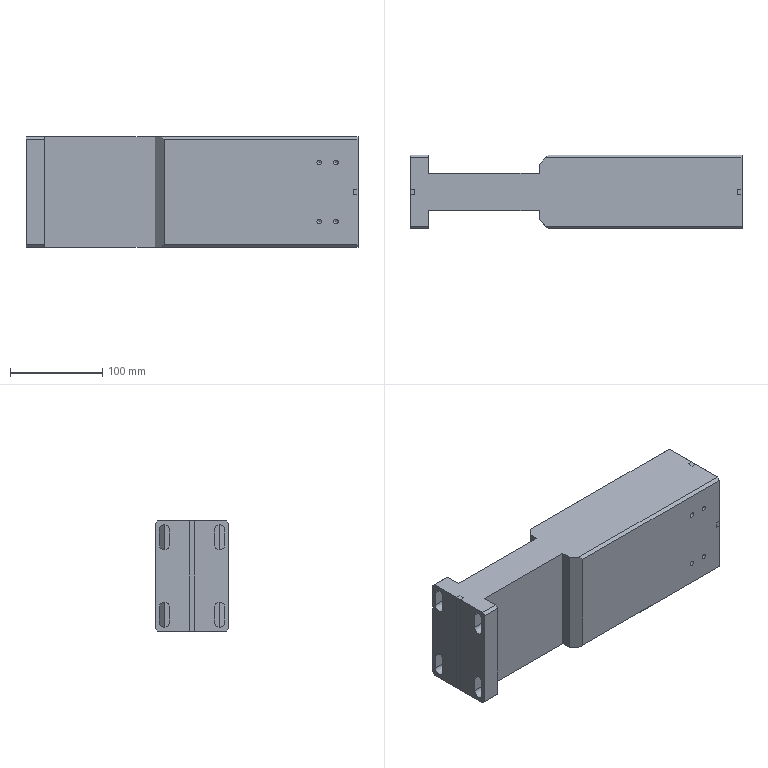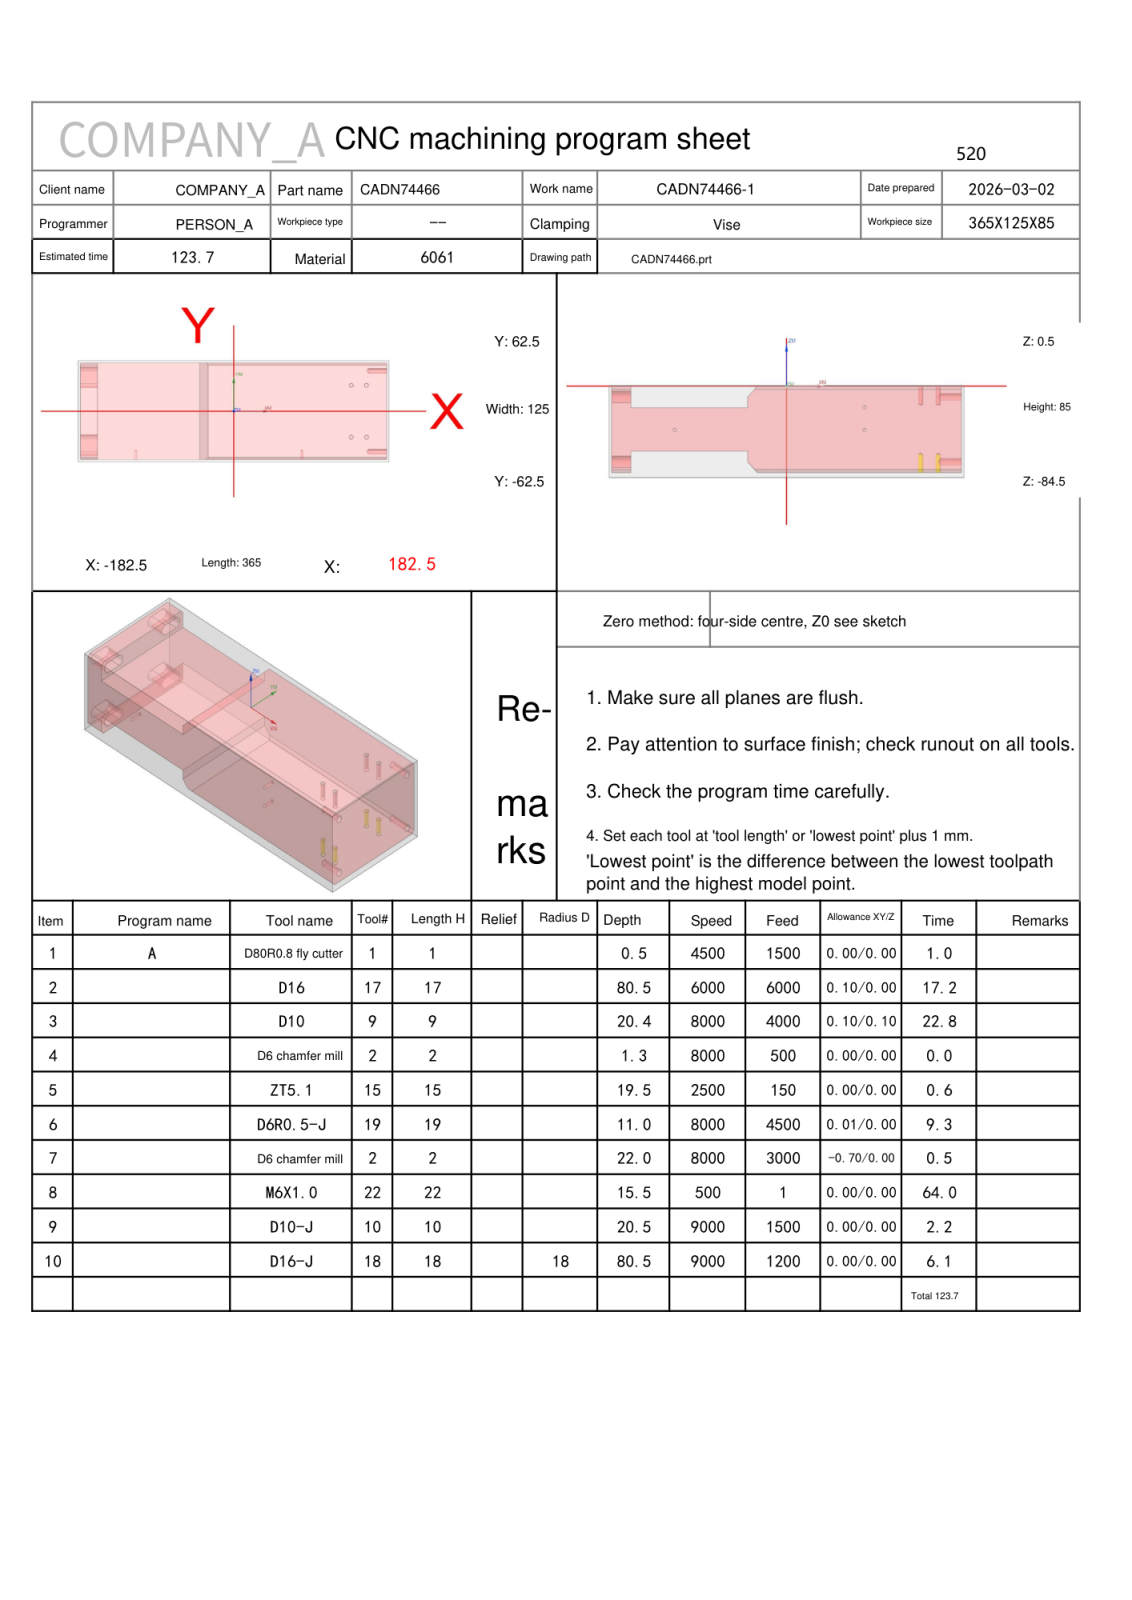NC program | NX | posted by the shop | part box 360 x 80 x 120 mm
Lines 5700 to 7747 of 7747:
N4 T02 M06
(D6 chamfer mill  D=6. R=0. H=02 ce=0.00 di=0.10)
G00 G90 G54 X138. Y32. M03 S8000
G43 H02 Z50.
M08
G98 G81 X138. Y32. Z-.8 R1. F500.
X156.
Y-32.
X138.
G80
G00 Z50.
G91 G28 Z0.0
M05
M09
G91 G28 Z0.0
M01
N5 T15 M06
(ZT5.1 D=5.1 DR_a=118 H=15)
G00 G90 G54 X138. Y32. M03 S2500
G43 H15 Z50.
M08
G98 G83 X138. Y32. Z-19. R1. F150. Q3.
X156.
Y-32.
X138.
G80
G00 Z50.
G91 G28 Z0.0
M05
M09
G91 G28 Z0.0
M01
N6 T19 M06
(D6R0.5-J  D=6. R=0.5 H=19 ce=0.01 di=0.00)
G00 G90 G54 X-32.786 Y-63.363 M03 S8000
G43 H19 Z10.788
M08
Z.429
G01 Z-.071 F4500.
Y-58.232
Y58.232
X-32.857 Y58.303 Z-.141
Y-58.303
X-32.927 Y-58.375 Z-.212
X-32.929 Y-58.275
Y58.275
X-32.927 Y58.375
X-32.996 Y58.446 Z-.283
X-33. Y58.275
Y-58.275
X-32.996 Y-58.446
X-33.068 Y-58.517 Z-.354
X-33.071 Y-58.275
Y58.275
X-33.068 Y58.517
X-33.14 Y58.588 Z-.424
X-33.141 Y57.278
Y-57.278
X-33.14 Y-58.588
X-33.21 Y-58.66 Z-.495
X-33.212 Y-58.622
Y58.622
X-33.21 Y58.66
X-33.28 Y58.731 Z-.566
X-33.283 Y58.622
Y-58.622
X-33.28 Y-58.731
X-33.35 Y-58.802 Z-.636
X-33.354 Y-58.622
Y58.622
X-33.35 Y58.802
X-33.421 Y58.873 Z-.707
X-33.424 Y58.622
Y-58.622
X-33.421 Y-58.873
X-33.494 Y-58.944 Z-.778
X-33.495 Y-57.631
Y57.631
X-33.494 Y58.944
X-33.563 Y59.015 Z-.849
X-33.566 Y58.969
Y-58.969
X-33.563 Y-59.015
X-33.633 Y-59.085 Z-.919
X-33.636 Y-58.969
Y58.969
X-33.633 Y59.085
X-33.704 Y59.156 Z-.99
X-33.707 Y58.969
Y-58.969
X-33.704 Y-59.156
X-33.775 Y-59.227 Z-1.061
X-33.778 Y-58.969
Y58.969
X-33.775 Y59.227
X-33.848 Y59.297 Z-1.131
Y57.985
Y-57.985
Y-59.297
X-33.917 Y-59.368 Z-1.202
X-33.919 Y-59.316
Y59.316
X-33.917 Y59.368
X-33.987 Y59.438 Z-1.273
X-33.99 Y59.316
Y-59.316
X-33.987 Y-59.438
X-34.057 Y-59.509 Z-1.344
X-34.061 Y-59.316
Y59.316
X-34.057 Y59.509
X-34.129 Y59.58 Z-1.414
X-34.131 Y58.268
Y-58.268
X-34.129 Y-59.58
X-34.202 Y-59.651 Z-1.485
Y-58.339
Y58.339
Y59.651
X-34.27 Y59.721 Z-1.556
X-34.273 Y59.663
Y-59.663
X-34.27 Y-59.721
X-34.34 Y-59.792 Z-1.626
X-34.343 Y-59.663
Y59.663
X-34.34 Y59.792
X-34.411 Y59.862 Z-1.697
X-34.414 Y59.663
Y-59.663
X-34.411 Y-59.862
X-34.482 Y-59.932 Z-1.768
X-34.485 Y-58.621
Y58.621
X-34.482 Y59.932
X-34.555 Y60.002 Z-1.838
X-34.556 Y58.692
Y-58.692
X-34.555 Y-60.002
X-34.624 Y-60.072 Z-1.909
X-34.626 Y-60.009
Y60.009
X-34.624 Y60.072
X-34.694 Y60.142 Z-1.98
X-34.697 Y60.009
Y-60.009
X-34.694 Y-60.142
X-34.764 Y-60.212 Z-2.051
X-34.768 Y-60.009
Y60.009
X-34.764 Y60.212
X-34.836 Y60.282 Z-2.121
X-34.838 Y58.975
Y-58.975
X-34.836 Y-60.282
X-34.909 Y-60.352 Z-2.192
Y-59.046
Y59.046
Y60.352
X-34.977 Y60.422 Z-2.263
X-34.98 Y60.356
Y-60.356
X-34.977 Y-60.422
X-35.047 Y-60.492 Z-2.333
X-35.051 Y-60.356
Y60.356
X-35.047 Y60.492
X-35.118 Y60.562 Z-2.404
X-35.121 Y60.356
Y-60.356
X-35.118 Y-60.562
X-35.19 Y-60.632 Z-2.475
X-35.192 Y-59.328
Y59.328
X-35.19 Y60.632
X-35.263 Y60.702 Z-2.546
Y59.399
Y-59.399
Y-60.702
X-35.331 Y-60.772 Z-2.616
X-35.333 Y-60.703
Y60.703
X-35.331 Y60.772
X-35.401 Y60.842 Z-2.687
X-35.404 Y60.703
Y-60.703
X-35.401 Y-60.842
X-35.471 Y-60.912 Z-2.758
X-35.475 Y-60.703
Y60.703
X-35.471 Y60.912
X-35.543 Y60.983 Z-2.828
X-35.546 Y59.682
Y-59.682
X-35.543 Y-60.982
X-35.616 Y-61.05 Z-2.899
Y-59.753
Y59.753
Y61.05
X-35.652 Y61.056 Z-2.934
X-35.686 Y61.061 Z-2.97
X-35.687 Y59.823
Y-59.823
X-35.686 Y-61.061
X-35.722 Y-61.062 Z-3.005
X-35.757 Z-3.041
X-35.758 Y-59.894
Y59.894
X-35.757 Y61.062
X-35.793 Y61.063 Z-3.076
X-35.828 Z-3.111
Y59.965
Y-59.965
Y-61.063
X-35.864 Y-61.064 Z-3.147
X-35.898 Z-3.182
X-35.899 Y-60.
Y60.
X-35.898 Y61.064
X-35.934 Z-3.217
X-35.969 Y61.065 Z-3.253
X-35.97 Y60.
Y-60.
X-35.969 Y-61.065
X-36.005 Z-3.288
X-36.04 Z-3.323
X-36.041 Y-60.
Y60.
X-36.04 Y61.065
X-36.076 Y61.066 Z-3.359
X-36.11 Z-3.394
X-36.111 Y60.
Y-60.
X-36.11 Y-61.066
X-36.147 Y-61.067 Z-3.429
X-36.181 Z-3.465
X-36.182 Y-60.
Y60.
X-36.181 Y61.067
X-36.217 Z-3.5
X-36.252 Y61.068 Z-3.536
X-36.253 Y60.
Y-60.
X-36.252 Y-61.068
X-36.288 Z-3.571
X-36.322 Z-3.606
X-36.323 Y-60.
Y60.
X-36.322 Y61.068
X-36.359 Y61.069 Z-3.642
X-36.393 Z-3.677
X-36.394 Y60.
Y-60.
X-36.393 Y-61.069
X-36.429 Z-3.712
X-36.464 Y-61.07 Z-3.748
X-36.465 Y-60.
Y60.
X-36.464 Y61.07
X-36.5 Z-3.783
X-36.534 Y61.071 Z-3.818
X-36.535 Y60.
Y-60.
X-36.534 Y-61.071
X-36.571 Z-3.854
X-36.605 Z-3.889
X-36.606 Y-60.
Y60.
X-36.605 Y61.071
X-36.642 Y61.072 Z-3.924
X-36.676 Z-3.96
X-36.677 Y60.
Y-60.
X-36.676 Y-61.072
X-36.712 Z-3.995
X-36.746 Y-61.073 Z-4.031
X-36.748 Y-60.
Y60.
X-36.746 Y61.073
X-36.783 Z-4.066
X-36.817 Y61.074 Z-4.101
X-36.818 Y60.
Y-60.
X-36.817 Y-61.073
X-36.854 Y-61.074 Z-4.137
X-36.888 Z-4.172
X-36.889 Y-60.
Y60.
X-36.888 Y61.074
X-36.924 Y61.075 Z-4.207
X-36.958 Z-4.243
X-36.96 Y61.05
Y-61.05
X-36.958 Y-61.075
X-36.995 Z-4.278
X-37.029 Y-61.076 Z-4.313
X-37.03 Y-61.05
Y61.05
X-37.029 Y61.076
X-37.066 Z-4.349
X-37.1 Z-4.384
X-37.101 Y61.05
Y-61.05
X-37.1 Y-61.076
X-37.137 Y-61.077 Z-4.419
X-37.17 Z-4.455
X-37.172 Y-61.05
Y61.05
X-37.17 Y61.077
X-37.207 Z-4.49
X-37.241 Y61.078 Z-4.525
X-37.243 Y61.05
Y-61.05
X-37.241 Y-61.078
X-37.278 Z-4.561
X-37.312 Z-4.596
X-37.313 Y-61.05
Y61.05
X-37.312 Y61.078
X-37.349 Y61.079 Z-4.632
X-37.383 Z-4.667
X-37.384 Y61.05
Y-61.05
X-37.383 Y-61.079
X-37.419 Z-4.702
X-37.453 Z-4.738
X-37.455 Y-61.05
Y61.05
X-37.453 Y61.079
X-37.49 Y61.08 Z-4.773
X-37.524 Z-4.808
X-37.525 Y61.05
Y-61.05
X-37.524 Y-61.08
X-37.561 Z-4.844
X-37.595 Z-4.879
X-37.596 Y-61.05
Y61.05
X-37.595 Y61.08
X-37.632 Y61.081 Z-4.914
X-37.665 Z-4.95
X-37.667 Y61.05
Y-61.05
X-37.665 Y-61.081
X-37.702 Z-4.985
X-37.736 Z-5.02
X-37.738 Y-61.05
Y61.05
X-37.736 Y61.081
X-37.773 Y61.082 Z-5.056
X-37.807 Z-5.091
X-37.808 Y61.05
Y-61.05
X-37.807 Y-61.082
X-37.844 Z-5.127
X-37.877 Z-5.162
X-37.879 Y-61.05
Y61.05
X-37.877 Y61.082
X-37.914 Y61.083 Z-5.197
X-37.948 Z-5.233
X-37.95 Y61.05
Y-61.05
X-37.948 Y-61.083
X-37.985 Z-5.268
X-38.019 Z-5.303
X-38.02 Y-61.05
Y61.05
X-38.019 Y61.083
X-38.056 Y61.084 Z-5.339
X-38.089 Z-5.374
X-38.091 Y61.05
Y-61.05
X-38.089 Y-61.084
X-38.126 Z-5.409
X-38.16 Z-5.445
X-38.162 Y-61.05
Y61.05
X-38.16 Y61.084
X-38.197 Z-5.48
X-38.231 Y61.085 Z-5.515
X-38.233 Y61.05
Y-61.05
X-38.231 Y-61.085
X-38.268 Z-5.551
X-38.302 Z-5.586
X-38.303 Y-61.05
Y61.05
X-38.302 Y61.085
X-38.339 Z-5.622
X-38.372 Y61.086 Z-5.657
X-38.374 Y61.05
Y-61.05
X-38.372 Y-61.086
X-38.409 Z-5.692
X-38.443 Z-5.728
X-38.445 Y-61.05
Y61.05
X-38.443 Y61.086
X-38.48 Z-5.763
X-38.514 Y61.087 Z-5.798
X-38.515 Y61.05
Y-61.05
X-38.514 Y-61.087
X-38.551 Z-5.834
X-38.584 Z-5.869
X-38.586 Y-61.05
Y61.05
X-38.584 Y61.087
X-38.621 Z-5.904
X-38.655 Z-5.94
X-38.657 Y61.05
Y-61.05
X-38.655 Y-61.087
X-38.692 Z-5.975
X-38.726 Z-6.01
X-38.728 Y-60.
Y61.05
X-38.726 Y61.088
X-38.763 Z-6.046
X-38.796 Z-6.081
X-38.798 Y61.05
Y-61.05
X-38.796 Y-61.088
X-38.834 Z-6.116
X-38.867 Z-6.152
X-38.869 Y-61.05
Y61.05
X-38.867 Y61.088
X-38.904 Z-6.187
X-38.938 Z-6.223
X-38.94 Y61.05
Y-61.05
X-38.938 Y-61.088
X-38.975 Z-6.258
X-39.009 Z-6.293
X-39.01 Y-61.05
Y61.05
X-39.009 Y61.088
X-39.046 Z-6.329
X-39.079 Z-6.364
X-39.081 Y61.05
Y-61.05
X-39.079 Y-61.088
X-39.116 Z-6.399
X-39.15 Z-6.435
X-39.152 Y-61.05
Y61.05
X-39.15 Y61.088
X-39.187 Z-6.47
X-39.221 Z-6.505
X-39.222 Y61.05
Y-61.05
X-39.221 Y-61.088
X-39.258 Z-6.541
X-39.291 Y-61.089 Z-6.576
X-39.293 Y-61.05
Y61.05
X-39.291 Y61.088
X-39.329 Z-6.611
X-39.362 Y61.089 Z-6.647
X-39.364 Y61.05
Y-61.05
X-39.362 Y-61.089
X-39.399 Z-6.682
X-39.433 Z-6.718
X-39.435 Y-61.05
Y61.05
X-39.433 Y61.089
X-39.47 Z-6.753
X-39.504 Z-6.788
X-39.505 Y61.05
Y-61.05
X-39.504 Y-61.089
X-39.541 Z-6.824
X-39.574 Z-6.859
X-39.576 Y-61.05
Y61.05
X-39.574 Y61.089
X-39.611 Z-6.894
X-39.645 Z-6.93
X-39.647 Y61.05
Y-61.05
X-39.645 Y-61.089
X-39.682 Z-6.965
X-39.716 Z-7.
X-39.717 Y-61.05
Y61.05
X-39.716 Y61.089
X-39.753 Z-7.036
X-39.786 Z-7.071
X-39.788 Y61.05
Y-61.05
X-39.786 Y-61.089
X-39.824 Z-7.106
X-39.857 Z-7.142
X-39.859 Y-61.05
Y61.05
X-39.857 Y61.089
X-39.894 Z-7.177
X-39.928 Z-7.212
X-39.93 Y61.05
Y-61.05
X-39.928 Y-61.089
X-39.965 Z-7.248
X-39.998 Z-7.283
X-40. Y-61.05
Y61.05
X-39.998 Y61.089
X-40.036 Z-7.319
X-40.069 Z-7.354
X-40.071 Y61.05
Y-61.05
X-40.069 Y-61.089
X-40.106 Z-7.389
X-40.14 Z-7.425
X-40.142 Y-61.05
Y61.05
X-40.14 Y61.089
X-40.177 Z-7.46
X-40.211 Z-7.495
X-40.212 Y61.05
Y-61.05
X-40.211 Y-61.089
X-40.248 Z-7.531
X-40.281 Z-7.566
X-40.283 Y-61.05
Y61.05
X-40.281 Y61.089
X-40.319 Z-7.601
X-40.352 Y61.088 Z-7.637
X-40.354 Y61.05
Y-61.05
X-40.352 Y-61.088
X-40.389 Z-7.672
X-40.423 Z-7.707
X-40.425 Y-61.05
Y61.05
X-40.423 Y61.088
X-40.46 Z-7.743
X-40.493 Z-7.778
X-40.495 Y61.05
Y-61.05
X-40.493 Y-61.088
X-40.531 Z-7.814
X-40.564 Z-7.849
X-40.566 Y-61.05
Y61.05
X-40.564 Y61.088
X-40.601 Z-7.884
X-40.635 Y61.087 Z-7.92
X-40.637 Y61.05
Y-61.05
X-40.635 Y-61.087
X-40.672 Z-7.955
X-40.706 Z-7.99
X-40.707 Y-61.05
Y61.05
X-40.706 Y61.087
X-40.743 Z-8.026
X-40.776 Z-8.061
X-40.778 Y61.05
Y-61.05
X-40.776 Y-61.087
X-40.813 Z-8.096
X-40.847 Y-61.086 Z-8.132
X-40.849 Y-61.05
Y61.05
X-40.847 Y61.087
X-40.884 Z-8.167
X-40.918 Y61.086 Z-8.202
X-40.92 Y61.05
Y-61.05
X-40.918 Y-61.086
X-40.955 Z-8.238
X-40.989 Z-8.273
X-40.99 Y-61.05
Y61.05
X-40.989 Y61.086
X-41.026 Z-8.309
X-41.059 Z-8.344
X-41.061 Y61.05
Y-61.05
X-41.059 Y-61.086
X-41.096 Z-8.379
X-41.13 Z-8.415
X-41.132 Y-61.05
Y61.05
X-41.13 Y61.086
X-41.167 Y61.085 Z-8.45
X-41.201 Z-8.485
X-41.202 Y61.05
Y-61.05
X-41.201 Y-61.085
X-41.238 Z-8.521
X-41.271 Z-8.556
X-41.273 Y-61.05
Y61.05
X-41.271 Y61.085
X-41.308 Z-8.591
X-41.342 Z-8.627
X-41.344 Y61.05
Y-61.05
X-41.342 Y-61.085
X-41.379 Z-8.662
X-41.413 Y-61.084 Z-8.697
X-41.415 Y-61.05
Y61.05
X-41.413 Y61.084
X-41.45 Z-8.733
X-41.484 Z-8.768
X-41.485 Y61.05
Y-61.05
X-41.484 Y-61.084
X-41.521 Z-8.803
X-41.554 Z-8.839
X-41.556 Y-61.05
Y61.05
X-41.554 Y61.084
X-41.591 Y61.083 Z-8.874
X-41.625 Z-8.91
X-41.627 Y61.05
Y-61.05
X-41.625 Y-61.083
X-41.662 Z-8.945
X-41.696 Z-8.98
X-41.697 Y-61.05
Y61.05
X-41.696 Y61.083
X-41.733 Y61.082 Z-9.016
X-41.766 Z-9.051
X-41.768 Y61.05
Y-61.05
X-41.766 Y-61.082
X-41.803 Z-9.086
X-41.837 Z-9.122
X-41.839 Y-61.05
Y61.05
X-41.837 Y61.082
X-41.874 Z-9.157
X-41.908 Y61.081 Z-9.192
X-41.909 Y61.05
Y-61.05
X-41.908 Y-61.081
X-41.945 Z-9.228
X-41.979 Z-9.263
X-41.98 Y-61.05
Y61.05
X-41.979 Y61.081
X-42.016 Z-9.298
X-42.049 Y61.08 Z-9.334
X-42.051 Y61.05
Y-61.05
X-42.049 Y-61.08
X-42.086 Z-9.369
X-42.12 Z-9.405
X-42.122 Y-61.05
Y61.05
X-42.12 Y61.08
X-42.157 Z-9.44
X-42.191 Y61.079 Z-9.475
X-42.192 Y61.05
Y-61.05
X-42.191 Y-61.079
X-42.228 Z-9.511
X-42.262 Z-9.546
X-42.263 Y-61.05
Y61.05
X-42.262 Y61.079
X-42.298 Z-9.581
X-42.332 Y61.078 Z-9.617
X-42.334 Y61.05
Y-61.05
X-42.332 Y-61.078
X-42.369 Z-9.652
X-42.403 Z-9.687
X-42.404 Y-61.05
Y61.05
X-42.403 Y61.078
X-42.44 Z-9.723
X-42.474 Y61.077 Z-9.758
X-42.475 Y61.05
Y-61.05
X-42.474 Y-61.078
X-42.511 Y-61.077 Z-9.793
X-42.545 Z-9.829
X-42.546 Y-61.05
Y61.05
X-42.545 Y61.077
X-42.581 Z-9.864
X-42.616 Y61.076 Z-9.899
X-42.617 Y60.
Y-60.
X-42.616 Y-61.077
X-42.652 Y-61.076 Z-9.935
X-42.686 Z-9.97
X-42.687 Y-61.05
Y61.05
X-42.686 Y61.076
X-42.723 Z-10.006
X-42.757 Z-10.041
X-42.758 Y61.05
Y-61.05
X-42.757 Y-61.076
X-42.793 Y-61.075 Z-10.076
X-42.827 Z-10.112
X-42.829 Y-61.05
Y61.05
X-42.827 Y61.075
X-42.864 Z-10.147
X-42.898 Z-10.182
Y-61.075
X-42.935 Y-61.074 Z-10.218
X-42.969 Z-10.253
Y61.074
X-43.001 Z-10.284
X-43.031 Z-10.315
Y-61.074
X-43.063 Z-10.346
X-43.092 Y-61.073 Z-10.377
Y61.073
X-43.125 Z-10.407
X-43.154 Z-10.438
Y-61.073
X-43.186 Z-10.469
X-43.216 Z-10.5
Y61.073
G00 Z10.788
G00 G90 X-153.773 Y-59.784 M03 S8000
Z10.788
Z.429
G01 Z-.071 F4500.
X-158.926 Y-59.785
X-181.074 Y-59.788
Y-59.823 Z-.106
Y-59.858 Z-.141
X-158.926 Y-59.856
Y-59.894 Z-.177
Y-59.926 Z-.212
X-159.076 Y-59.929
X-180.
X-181.074
X-181.075 Y-59.965 Z-.247
Y-60. Z-.283
X-180.
X-159.076
X-158.925 Y-59.997
Y-60.035 Z-.318
Y-60.068 Z-.354
X-159.076 Y-60.071
X-180.
X-181.075
Y-60.106 Z-.389
X-181.076 Y-60.141 Z-.424
X-180.
X-159.076
X-158.924 Y-60.139
Y-60.177 Z-.46
Y-60.209 Z-.495
X-159.076 Y-60.212
X-180.
X-181.076
Y-60.247 Z-.53
Y-60.283 Z-.566
X-180.
X-159.076
X-158.924 Y-60.28
Y-60.318 Z-.601
X-158.923 Y-60.351 Z-.636
X-159.076 Y-60.354
X-180.
X-181.077 Y-60.353
Y-60.389 Z-.672
Y-60.424 Z-.707
X-180.
X-159.076
X-158.923 Y-60.421
Y-60.46 Z-.742
Y-60.492 Z-.778
X-159.076 Y-60.495
X-180.
X-181.077
X-181.078 Y-60.53 Z-.813
Y-60.566 Z-.849
X-180.
X-159.076
X-158.922 Y-60.563
Y-60.601 Z-.884
Y-60.634 Z-.919
X-159.076 Y-60.636
X-180.
X-181.078
Y-60.672 Z-.955
Y-60.707 Z-.99
X-180.
X-159.076
X-158.922 Y-60.704
X-158.921 Y-60.742 Z-1.025
Y-60.775 Z-1.061
X-159.076 Y-60.778
X-180.
X-181.079
Y-60.813 Z-1.096
Y-60.848 Z-1.131
X-180.
X-159.076
X-158.921 Y-60.846
Y-60.884 Z-1.167
Y-60.916 Z-1.202
X-159.076 Y-60.919
X-180.
X-181.079
Y-60.955 Z-1.237
Y-60.99 Z-1.273
X-180.
X-159.076
X-158.921 Y-60.987
Y-61.025 Z-1.308
Y-61.058 Z-1.344
X-159.076 Y-61.061
X-180.
X-181.079
Y-61.096 Z-1.379
Y-61.131 Z-1.414
X-180.
X-160.
X-158.921
Y-61.167 Z-1.45
Y-61.199 Z-1.485
X-159.076 Y-61.202
X-180.
X-181.079
Y-61.237 Z-1.52
Y-61.273 Z-1.556
X-180.
X-159.076
X-158.921 Y-61.27
Y-61.308 Z-1.591
Y-61.341 Z-1.626
X-159.076 Y-61.343
X-180.
X-181.079
Y-61.379 Z-1.662
Y-61.414 Z-1.697
X-180.
X-159.076
X-158.921 Y-61.411
Y-61.45 Z-1.732
Y-61.482 Z-1.768
X-159.076 Y-61.485
X-180.
X-181.079
Y-61.52 Z-1.803
Y-61.556 Z-1.838
X-180.
X-159.076
X-158.921 Y-61.553
Y-61.591 Z-1.874
Y-61.623 Z-1.909
X-159.076 Y-61.626
X-180.
X-181.079
Y-61.662 Z-1.945
Y-61.697 Z-1.98
X-180.
X-159.076
X-158.921 Y-61.694
Y-61.732 Z-2.015
Y-61.765 Z-2.051
X-159.076 Y-61.768
X-180.
X-181.079
Y-61.803 Z-2.086
Y-61.838 Z-2.121
X-180.
X-159.076
X-158.921 Y-61.836
Y-61.874 Z-2.157
Y-61.906 Z-2.192
X-159.076 Y-61.909
X-180.
X-181.079
Y-61.944 Z-2.227
Y-61.98 Z-2.263
X-180.
X-159.076
X-158.922 Y-61.977
Y-62.015 Z-2.298
Y-62.048 Z-2.333
X-159.076 Y-62.051
X-180.
X-181.078
Y-62.086 Z-2.369
Y-62.121 Z-2.404
X-180.
X-159.076
X-158.922 Y-62.118
Y-62.157 Z-2.44
Y-62.189 Z-2.475
X-159.076 Y-62.192
X-180.
X-181.078
X-181.077 Y-62.227 Z-2.51
Y-62.263 Z-2.546
X-180.
X-159.076
X-158.923 Y-62.26
Y-62.298 Z-2.581
Y-62.331 Z-2.616
X-159.076 Y-62.333
X-180.
X-181.077
Y-62.369 Z-2.652
X-181.076 Y-62.404 Z-2.687
X-180.
X-159.076
X-158.924 Y-62.401
Y-62.439 Z-2.722
Y-62.472 Z-2.758
X-159.076 Y-62.475
X-180.
X-181.076
Y-62.51 Z-2.793
Y-62.545 Z-2.828
X-180. Y-62.546
X-159.076
X-158.924 Y-62.543
X-158.925 Y-62.581 Z-2.864
Y-62.613 Z-2.899
X-159.076 Y-62.616
X-180.
X-181.075
Y-62.652 Z-2.934
Y-62.687 Z-2.97
X-180.
X-159.076
X-158.925 Y-62.684
Y-62.722 Z-3.005
X-158.926 Y-62.755 Z-3.041
X-159.076 Y-62.758
X-180.
X-181.075
X-181.074 Y-62.793 Z-3.076
Y-62.828 Z-3.111
X-180.
X-159.076
X-158.926 Y-62.826
Y-62.864 Z-3.147
Y-62.896 Z-3.182
X-181.074 Y-62.899
Y-62.934 Z-3.217
X-181.073 Y-62.97 Z-3.253
X-158.927 Y-62.967
Y-63.001 Z-3.284
Y-63.029 Z-3.315
X-181.073 Y-63.032
Y-63.063 Z-3.345
Y-63.093 Z-3.376
X-158.927 Y-63.091
Y-63.124 Z-3.407
X-158.928 Y-63.152 Z-3.438
X-181.073 Y-63.155
X-181.072 Y-63.186 Z-3.469
Y-63.217 Z-3.5
X-158.928 Y-63.214
G00 Z10.788
X-186.221 Y59.788
Z.429
G01 Z-.071
X-181.074
X-158.926 Y59.785
Y59.823 Z-.106
Y59.856 Z-.141
X-181.074 Y59.858
Y59.894 Z-.177
Y59.929 Z-.212
X-180.
X-159.076
X-158.926 Y59.926
X-158.925 Y59.965 Z-.247
Y59.997 Z-.283
X-159.076 Y60.
X-180.
X-181.075
Y60.035 Z-.318
Y60.071 Z-.354
X-180.
X-159.076
X-158.925 Y60.068
Y60.106 Z-.389
X-158.924 Y60.139 Z-.424
X-159.076 Y60.141
X-180.
X-181.076
Y60.177 Z-.46
Y60.212 Z-.495
X-180.
X-159.076
X-158.924 Y60.209
Y60.247 Z-.53
Y60.28 Z-.566
X-159.076 Y60.283
X-180.
X-181.076
X-181.077 Y60.318 Z-.601
Y60.353 Z-.636
X-180. Y60.354
X-159.076
X-158.923 Y60.351
Y60.389 Z-.672
Y60.421 Z-.707
X-159.076 Y60.424
X-180.
X-181.077
Y60.46 Z-.742
Y60.495 Z-.778
X-180.
X-159.076
X-158.923 Y60.492
X-158.922 Y60.53 Z-.813
Y60.563 Z-.849
X-159.076 Y60.566
X-180.
X-181.078
Y60.601 Z-.884
Y60.636 Z-.919
X-180.
X-159.076
X-158.922 Y60.634
Y60.672 Z-.955
Y60.704 Z-.99
X-159.076 Y60.707
X-180.
X-181.078
X-181.079 Y60.742 Z-1.025
Y60.778 Z-1.061
X-180.
X-159.076
X-158.921 Y60.775
Y60.813 Z-1.096
Y60.846 Z-1.131
X-159.076 Y60.848
X-180.
X-181.079
Y60.884 Z-1.167
Y60.919 Z-1.202
X-180.
X-159.076
X-158.921 Y60.916
Y60.955 Z-1.237
Y60.987 Z-1.273
X-159.076 Y60.99
X-180.
X-181.079
Y61.025 Z-1.308
Y61.061 Z-1.344
X-180.
X-159.076
X-158.921 Y61.058
Y61.096 Z-1.379
Y61.131 Z-1.414
X-160.
X-180.
X-181.079
Y61.167 Z-1.45
Y61.202 Z-1.485
X-180.
X-159.076
X-158.921 Y61.199
Y61.237 Z-1.52
Y61.27 Z-1.556
X-159.076 Y61.273
X-180.
X-181.079
Y61.308 Z-1.591
Y61.343 Z-1.626
X-180.
X-159.076
X-158.921 Y61.341
Y61.379 Z-1.662
Y61.411 Z-1.697
X-159.076 Y61.414
X-180.
X-181.079
Y61.45 Z-1.732
Y61.485 Z-1.768
X-180.
X-159.076
X-158.921 Y61.482
Y61.52 Z-1.803
Y61.553 Z-1.838
X-159.076 Y61.556
X-180.
X-181.079
Y61.591 Z-1.874
Y61.626 Z-1.909
X-180.
X-159.076
X-158.921 Y61.623
Y61.662 Z-1.945
Y61.694 Z-1.98
X-159.076 Y61.697
X-180.
X-181.079
Y61.732 Z-2.015
Y61.768 Z-2.051
X-180.
X-159.076
X-158.921 Y61.765
Y61.803 Z-2.086
Y61.836 Z-2.121
X-159.076 Y61.838
X-180.
X-181.079
Y61.874 Z-2.157
Y61.909 Z-2.192
X-180.
X-159.076
X-158.921 Y61.906
Y61.944 Z-2.227
X-158.922 Y61.977 Z-2.263
X-159.076 Y61.98
X-180.
X-181.079
X-181.078 Y62.015 Z-2.298
Y62.051 Z-2.333
X-180.
X-159.076
X-158.922 Y62.048
Y62.086 Z-2.369
Y62.118 Z-2.404
X-159.076 Y62.121
X-180.
X-181.078
Y62.157 Z-2.44
Y62.192 Z-2.475
X-180.
X-159.076
X-158.922 Y62.189
X-158.923 Y62.227 Z-2.51
Y62.26 Z-2.546
X-159.076 Y62.263
X-180.
X-181.077
Y62.298 Z-2.581
Y62.333 Z-2.616
X-180.
X-159.076
X-158.923 Y62.331
Y62.369 Z-2.652
X-158.924 Y62.401 Z-2.687
X-159.076 Y62.404
X-180.
X-181.076
Y62.439 Z-2.722
Y62.475 Z-2.758
X-180.
X-159.076
X-158.924 Y62.472
Y62.51 Z-2.793
Y62.543 Z-2.828
X-159.076 Y62.546
X-180.
X-181.076 Y62.545
X-181.075 Y62.581 Z-2.864
Y62.616 Z-2.899
X-180.
X-159.076
X-158.925 Y62.613
Y62.652 Z-2.934
Y62.684 Z-2.97
X-159.076 Y62.687
X-180.
X-181.075
Y62.722 Z-3.005
Y62.758 Z-3.041
X-180.
X-159.076
X-158.926 Y62.755
Y62.793 Z-3.076
Y62.826 Z-3.111
X-159.076 Y62.828
X-180.
X-181.074
Y62.864 Z-3.147
Y62.899 Z-3.182
X-158.926 Y62.896
Y62.934 Z-3.217
X-158.927 Y62.967 Z-3.253
X-181.073 Y62.97
Y63.001 Z-3.284
Y63.032 Z-3.315
X-158.927 Y63.029
Y63.063 Z-3.345
Y63.091 Z-3.376
X-181.073 Y63.093
Y63.124 Z-3.407
Y63.155 Z-3.438
X-158.928 Y63.152
Y63.186 Z-3.469
Y63.214 Z-3.5
X-181.072 Y63.217
G00 Z10.788
X-36.361 Y59.785
Z.429
G01 Z-.071
X-31.233
X181.074 Y59.787
Y59.823 Z-.106
Y59.857 Z-.141
X-31.304 Y59.855
X-31.376 Y59.927 Z-.212
X-30.066 Y59.929
X180.
X181.074 Y59.928
X181.075 Y59.965 Z-.247
Y59.999 Z-.283
X180. Y60.
X-30.136
X-31.447
X-31.518 Y60.068 Z-.354
X-31.447 Y60.071
X180.
X181.075 Y60.069
Y60.106 Z-.389
Y60.14 Z-.424
X180. Y60.141
X-31.447
X-31.59 Y60.138
X-31.661 Y60.209 Z-.495
X-31.447 Y60.212
X180.
X181.076 Y60.211
Y60.247 Z-.53
Y60.282 Z-.566
X180. Y60.283
X-30.419
X-31.733 Y60.281
X-31.804 Y60.353 Z-.636
X-30.49 Y60.354
X180.
X181.076 Y60.352
X181.077 Y60.389 Z-.672
Y60.423 Z-.707
X180. Y60.424
X-31.793
X-31.875 Y60.421
X-31.946 Y60.492 Z-.778
X-31.793 Y60.495
X180.
X181.077 Y60.494
Y60.53 Z-.813
X181.078 Y60.564 Z-.849
X180. Y60.566
X-31.793
X-32.017 Y60.563
X-32.088 Y60.635 Z-.919
X-30.773 Y60.636
X181.053
X181.078 Y60.635
Y60.672 Z-.955
Y60.706 Z-.99
X181.053 Y60.707
X-30.844
X-32.158 Y60.706
X-32.229 Y60.775 Z-1.061
X-32.14 Y60.778
X181.053
X181.079 Y60.776
Y60.813 Z-1.096
Y60.847 Z-1.131
X181.053 Y60.848
X-32.14
X-32.3 Y60.845
X-32.371 Y60.916 Z-1.202
X-32.14 Y60.919
X181.053
X181.079 Y60.918
Y60.955 Z-1.237
Y60.989 Z-1.273
X181.053 Y60.99
X-31.126
X-32.442 Y60.988
X-32.512 Y61.059 Z-1.344
X-32.487 Y61.061
X181.053
X181.079 Y61.059
Y61.096 Z-1.379
Y61.131 Z-1.414
X180.
X-31.268
X-32.583
X-32.654 Y61.199 Z-1.485
X-32.487 Y61.202
X181.053
X181.079 Y61.201
Y61.237 Z-1.52
Y61.271 Z-1.556
X181.053 Y61.273
X-32.487
X-32.725 Y61.27
X-32.796 Y61.342 Z-1.626
X-31.48 Y61.343
X181.053
X181.079 Y61.342
Y61.379 Z-1.662
Y61.413 Z-1.697
X181.053 Y61.414
X-32.833
X-32.866 Y61.412
X-32.937 Y61.482 Z-1.768
X-32.833 Y61.485
X181.053
X181.079 Y61.484
Y61.52 Z-1.803
Y61.554 Z-1.838
X181.053 Y61.556
X-32.833
X-33.007 Y61.552
X-33.077 Y61.623 Z-1.909
X-32.833 Y61.626
X181.053
X181.079 Y61.625
Y61.662 Z-1.945
Y61.696 Z-1.98
X181.053 Y61.697
X-31.833
X-33.147 Y61.696
X-33.217 Y61.766 Z-2.051
X-33.18 Y61.768
X181.053
X181.079 Y61.766
Y61.803 Z-2.086
Y61.837 Z-2.121
X181.053 Y61.838
X-33.18
X-33.288 Y61.835
X-33.358 Y61.906 Z-2.192
X-33.18 Y61.909
X181.053
X181.079 Y61.908
Y61.944 Z-2.227
X181.078 Y61.979 Z-2.263
X181.053 Y61.98
X-33.18
X-33.428 Y61.977
X-33.498 Y62.049 Z-2.333
X-32.187 Y62.051
X181.053
X181.078 Y62.049
Y62.086 Z-2.369
Y62.12 Z-2.404
X181.053 Y62.121
X-33.527
X-33.569 Y62.119
X-33.639 Y62.189 Z-2.475
X-33.527 Y62.192
X180.
X181.077 Y62.191
Y62.227 Z-2.51
Y62.261 Z-2.546
X180. Y62.263
X-33.527
X-33.709 Y62.259
X-33.779 Y62.33 Z-2.616
X-33.527 Y62.333
X180.
X181.077 Y62.332
Y62.369 Z-2.652
X181.076 Y62.403 Z-2.687
X180. Y62.404
X-32.541
X-33.85 Y62.403
X-33.92 Y62.473 Z-2.758
X-33.873 Y62.475
X180.
X181.076 Y62.474
Y62.51 Z-2.793
Y62.544 Z-2.828
X180. Y62.546
X-33.873
X-33.99 Y62.542
X-34.06 Y62.612 Z-2.899
X-33.873 Y62.616
X180.
X181.075 Y62.615
Y62.652 Z-2.934
Y62.686 Z-2.97
X180. Y62.687
X-33.873
X-34.13 Y62.684
X-34.201 Y62.757 Z-3.041
X-32.894 Y62.758
X180.
X181.075 Y62.757
X181.074 Y62.793 Z-3.076
Y62.827 Z-3.111
X180. Y62.828
X-34.22
X-34.271 Y62.826
X-34.246 Y62.898 Z-3.182
X181.074
Y62.934 Z-3.217
X181.073 Y62.969 Z-3.253
X-34.198
X-34.136 Y63.029 Z-3.315
X181.073 Y63.031
Y63.063 Z-3.345
Y63.092 Z-3.376
X-34.075 Y63.09
X-34.013 Y63.152 Z-3.438
X181.072 Y63.154
Y63.186 Z-3.469
Y63.216 Z-3.5
X-33.951 Y63.214
G00 Z10.788
X186.223 Y-59.787
Z.429
G01 Z-.071
X181.074
X-31.233 Y-59.785
X-31.304 Y-59.855 Z-.141
X181.074 Y-59.857
Y-59.894 Z-.177
Y-59.928 Z-.212
X180. Y-59.929
X-30.066
X-31.376 Y-59.927
X-31.447 Y-60. Z-.283
X-30.136
X180.
X181.075 Y-59.999
Y-60.035 Z-.318
Y-60.069 Z-.354
X180. Y-60.071
X-31.447
X-31.518 Y-60.068
X-31.59 Y-60.138 Z-.424
X-31.447 Y-60.141
X180.
X181.075 Y-60.14
X181.076 Y-60.177 Z-.46
Y-60.211 Z-.495
X180. Y-60.212
X-31.447
X-31.661 Y-60.209
X-31.733 Y-60.281 Z-.566
X-30.419 Y-60.283
X180.
X181.076 Y-60.282
Y-60.318 Z-.601
Y-60.352 Z-.636
X180. Y-60.354
X-30.49
X-31.804 Y-60.353
X-31.875 Y-60.421 Z-.707
X-31.793 Y-60.424
X180.
X181.077 Y-60.423
Y-60.46 Z-.742
Y-60.494 Z-.778
X180. Y-60.495
X-31.793
X-31.946 Y-60.492
X-32.017 Y-60.563 Z-.849
X-31.793 Y-60.566
X180.
X181.078 Y-60.564
Y-60.601 Z-.884
Y-60.635 Z-.919
X181.053 Y-60.636
X-30.773
X-32.088 Y-60.635
X-32.158 Y-60.706 Z-.99
X-30.844 Y-60.707
X181.053
X181.078 Y-60.706
X181.079 Y-60.742 Z-1.025
Y-60.776 Z-1.061
X181.053 Y-60.778
X-32.14
X-32.229 Y-60.775
X-32.3 Y-60.845 Z-1.131
X-32.14 Y-60.848
X181.053
X181.079 Y-60.847
Y-60.884 Z-1.167
Y-60.918 Z-1.202
X181.053 Y-60.919
X-32.14
X-32.371 Y-60.916
X-32.442 Y-60.988 Z-1.273
X-31.126 Y-60.99
X181.053
X181.079 Y-60.989
Y-61.025 Z-1.308
Y-61.059 Z-1.344
X181.053 Y-61.061
X-32.487
X-32.512 Y-61.059
X-32.583 Y-61.131 Z-1.414
X-31.268
X180.94
X181.08 Y-61.13
Y-61.167 Z-1.45
X181.079 Y-61.201 Z-1.485
X181.053 Y-61.202
X-32.487
X-32.654 Y-61.199
X-32.725 Y-61.27 Z-1.556
X-32.487 Y-61.273
X181.053
X181.079 Y-61.271
Y-61.308 Z-1.591
Y-61.342 Z-1.626
X181.053 Y-61.343
X-31.48
X-32.796 Y-61.342
X-32.866 Y-61.412 Z-1.697
X-32.833 Y-61.414
X181.053
X181.079 Y-61.413
Y-61.45 Z-1.732
Y-61.484 Z-1.768
X181.053 Y-61.485
X-32.833
X-32.937 Y-61.482
X-33.007 Y-61.552 Z-1.838
X-32.833 Y-61.556
X181.053
X181.079 Y-61.554
Y-61.591 Z-1.874
Y-61.625 Z-1.909
X181.053 Y-61.626
X-32.833
X-33.077 Y-61.623
X-33.147 Y-61.696 Z-1.98
X-31.833 Y-61.697
X181.053
X181.079 Y-61.696
Y-61.732 Z-2.015
Y-61.766 Z-2.051
X181.053 Y-61.768
X-33.18
X-33.217 Y-61.766
X-33.288 Y-61.835 Z-2.121
X-33.18 Y-61.838
X181.053
X181.079 Y-61.837
Y-61.874 Z-2.157
Y-61.908 Z-2.192
X181.053 Y-61.909
X-33.18
X-33.358 Y-61.906
X-33.428 Y-61.977 Z-2.263
X-33.18 Y-61.98
X181.053
X181.078 Y-61.979
Y-62.015 Z-2.298
Y-62.049 Z-2.333
X181.053 Y-62.051
X-32.187
X-33.498 Y-62.049
X-33.569 Y-62.119 Z-2.404
X-33.527 Y-62.121
X181.053
X181.078 Y-62.12
Y-62.157 Z-2.44
X181.077 Y-62.191 Z-2.475
X180. Y-62.192
X-33.527
X-33.639 Y-62.189
X-33.709 Y-62.259 Z-2.546
X-33.527 Y-62.263
X180.
X181.077 Y-62.261
Y-62.298 Z-2.581
Y-62.332 Z-2.616
X180. Y-62.333
X-33.527
X-33.779 Y-62.33
X-33.85 Y-62.403 Z-2.687
X-32.541 Y-62.404
X180.
X181.076 Y-62.403
Y-62.439 Z-2.722
Y-62.474 Z-2.758
X180. Y-62.475
X-33.873
X-33.92 Y-62.473
X-33.99 Y-62.542 Z-2.828
X-33.873 Y-62.546
X180.
X181.076 Y-62.544
X181.075 Y-62.581 Z-2.864
Y-62.615 Z-2.899
X180. Y-62.616
X-33.873
X-34.06 Y-62.612
X-34.13 Y-62.684 Z-2.97
X-33.873 Y-62.687
X180.
X181.075 Y-62.686
Y-62.722 Z-3.005
Y-62.757 Z-3.041
X180. Y-62.758
X-32.894
X-34.201 Y-62.757
X-34.271 Y-62.826 Z-3.111
X-34.22 Y-62.828
X180.
X181.074 Y-62.827
Y-62.864 Z-3.147
Y-62.898 Z-3.182
X-34.246
X-34.198 Y-62.969 Z-3.253
X181.073
Y-63.001 Z-3.284
Y-63.031 Z-3.315
X-34.136 Y-63.029
X-34.075 Y-63.09 Z-3.376
X181.073 Y-63.092
X181.072 Y-63.124 Z-3.407
Y-63.154 Z-3.438
X-34.013 Y-63.152
X-33.951 Y-63.214 Z-3.5
X181.072 Y-63.216
G00 Z10.788
G91 G28 Z0.0
M05
M09
G91 G28 Z0.0
M01
N7 T02 M06
(D6 chamfer mill  D=6. R=0. H=02 ce=0.00 di=0.00)
G00 G90 G54 X-181.207 Y-57.461 M03 S8000
G43 H02 Z50.
M08
Z2.935
G01 Z-1.5 F3000.
X-181.267 Y-57.289
X-181.3 Y-57.
Y57.
X-181.267 Y57.289
X-181.207 Y57.461
Z2.935
G00 Z50.
X-158.793
Z2.935
G01 Z-1.5
X-158.733 Y57.289
X-158.7 Y57.
Y0.0
Y-57.
X-158.733 Y-57.289
X-158.793 Y-57.461
Z2.935
G00 Z50.
X181.207 Y57.461
Z2.935
G01 Z-1.5
X181.267 Y57.289
X181.3 Y57.
Y-57.
X181.267 Y-57.289
X181.207 Y-57.461
Z2.935
G00 Z50.
X-43.032 Y-62.128
Z-7.184
G01 Z-21.5
G03 X-42.951 Y-61.828 I-.52 J.3
X-43.251 Y-61.308 I-.6 J0.0
G01 X-43.281 Y-61.3
X-156.719
X-156.749 Y-61.308
G03 X-157.049 Y-61.828 I.3 J-.52
X-156.968 Y-62.128 I.6 J0.0
G01 Z-.177
G00 Z50.
Y62.128
Z-.177
G01 Z-21.5
G03 X-157.049 Y61.828 I.52 J-.3
X-156.749 Y61.308 I.6 J0.0
G01 X-156.719 Y61.3
X-43.281
X-43.251 Y61.308
G03 X-42.951 Y61.828 I-.3 J.52
X-43.032 Y62.128 I-.6 J0.0
G01 Z-7.184
G00 Z50.
G00 G90 X155.13 Y-32.232 M03 S8000
Z50.
Z-.8
G01 Z-1.3 F600.
X154.5 Y-32.4
G03 X156. Y-33.9 I1.5 J0.0
X157.9 Y-32. I0.0 J1.9
X156. Y-30.1 I-1.9 J0.0
X154.1 Y-32. I0.0 J-1.9
X156. Y-33.9 I1.9 J0.0
X157.5 Y-32.4 I0.0 J1.5
G01 X156.87 Y-32.232
Z-.8
G00 Z50.
X137.13
Z-.8
G01 Z-1.3
X136.5 Y-32.4
G03 X138. Y-33.9 I1.5 J0.0
X139.9 Y-32. I0.0 J1.9
X138. Y-30.1 I-1.9 J0.0
X136.1 Y-32. I0.0 J-1.9
X138. Y-33.9 I1.9 J0.0
X139.5 Y-32.4 I0.0 J1.5
G01 X138.87 Y-32.232
Z-.8
G00 Z50.
X137.13 Y31.768
Z-.8
G01 Z-1.3
X136.5 Y31.6
G03 X138. Y30.1 I1.5 J0.0
X139.9 Y32. I0.0 J1.9
X138. Y33.9 I-1.9 J0.0
X136.1 Y32. I0.0 J-1.9
X138. Y30.1 I1.9 J0.0
X139.5 Y31.6 I0.0 J1.5
G01 X138.87 Y31.768
Z-.8
G00 Z50.
X155.13
Z-.8
G01 Z-1.3
X154.5 Y31.6
G03 X156. Y30.1 I1.5 J0.0
X157.9 Y32. I0.0 J1.9
X156. Y33.9 I-1.9 J0.0
X154.1 Y32. I0.0 J-1.9
X156. Y30.1 I1.9 J0.0
X157.5 Y31.6 I0.0 J1.5
G01 X156.87 Y31.768
Z-.8
G00 Z50.
G91 G28 Z0.0
M05
M09
G91 G28 Z0.0
M01
N8 T22 M06
(M6X1.0 D=5. DR_a=180 H=22)
G00 G90 G54 X138. Y32. M03 S500
G43 H22 Z50.
M08
G95
G98 G84 X138. Y32. Z-15. R1. F1. Q3.
X156.
Y-32.
X138.
G80
G94
G00 Z50.
G91 G28 Z0.0
M05
M09
G91 G28 Z0.0
M01
N9 T10 M06
(D10-J  D=10. R=0. H=10 ce=0.30 di=0.00)
G00 G90 G54 X-100. Y68. M03 S9000
G43 H10 Z50.
M08
Z-19.5
G01 Z-20. F1500.
Y61.
X-45.3
Y-61.
X-154.7
Y61.
X-100.
Y54.
X-52.3
Y-54.
X-147.7
Y54.
X-100.
Y47.
X-59.3
Y-47.
X-140.7
Y47.
X-100.
Y40.
X-66.3
Y-40.
X-133.7
Y40.
X-100.
Y33.
X-73.3
Y-33.
X-126.7
Y33.
X-100.
Y26.
X-80.3
Y-26.
X-119.7
Y26.
X-100.
Y19.
X-87.3
Y-19.
X-112.7
Y19.
X-100.
Y12.
X-94.3
Y-12.
X-105.7
Y12.
X-100.
Y7.5
X-98.8
Y-7.5
X-101.2
Y7.5
X-100.
X-99.5
Y13.5
Z-19.5
G00 Z50.
G00 G90 X-46.1 Y-65.5 M03 S9000
Z50.
Z-6.165
G01 Z-6.665 F1500.
G41 D10
X-46.
G03 X-45. Y-64.5 I0.0 J1.
G01 Y64.5
G03 X-46. Y65.5 I-1. J0.0
G01 G40 X-46.1
Z-6.165
G00 Z50.
Y-65.5
Z-12.83
G01 Z-13.33
G41 D10
X-46.
G03 X-45. Y-64.5 I0.0 J1.
G01 Y64.5
G03 X-46. Y65.5 I-1. J0.0
G01 G40 X-46.1
Z-12.83
G00 Z50.
X-153.9
Z-6.165
G01 Z-6.665
G41 D10
X-154.
G03 X-155. Y64.5 I0.0 J-1.
G01 Y-64.5
G03 X-154. Y-65.5 I1. J0.0
G01 G40 X-153.9
Z-6.165
G00 Z50.
Y65.5
Z-12.83
G01 Z-13.33
G41 D10
X-154.
G03 X-155. Y64.5 I0.0 J-1.
G01 Y-64.5
G03 X-154. Y-65.5 I1. J0.0
G01 G40 X-153.9
Z-12.83
G00 Z50.
X-46.1
Z-19.495
G01 Z-19.995
G41 D10
X-46.
G03 X-45. Y-64.5 I0.0 J1.
G01 Y64.5
G03 X-46. Y65.5 I-1. J0.0
G01 G40 X-46.1
Z-19.495
G00 Z50.
X-153.9
Z-19.495
G01 Z-19.995
G41 D10
X-154.
G03 X-155. Y64.5 I0.0 J-1.
G01 Y-64.5
G03 X-154. Y-65.5 I1. J0.0
G01 G40 X-153.9
Z-19.495
G00 Z50.
G91 G28 Z0.0
M05
M09
G91 G28 Z0.0
M01
N10 T18 M06
(D16-J  D=16. R=0. H=18 ce=0.00 di=0.00)
G00 G90 G54 X181.01 Y-69.144 M03 S9000
G43 H18 Z50.
M08
Z-10.929
G01 Z-11.429 F1200.
G41 D18
X180.998 Y-68.944
G03 X180. Y-68. I-.998 J-.056
G01 X-180.
G02 X-188. Y-60. I0.0 J8.
G01 Y60.
G02 X-180. Y68. I8. J0.0
G01 X180.
G02 X188. Y60. I0.0 J-8.
G01 Y-60.
G02 X180. Y-68. I-8. J0.0
G01 X179.5
G03 X178.5 Y-69. I0.0 J-1.
G01 G40 Y-69.2
Z-10.929
G00 Z50.
X181.01 Y-69.144
Z-22.357
G01 Z-22.857
G41 D18
X180.998 Y-68.944
G03 X180. Y-68. I-.998 J-.056
G01 X-180.
G02 X-188. Y-60. I0.0 J8.
G01 Y60.
G02 X-180. Y68. I8. J0.0
G01 X180.
G02 X188. Y60. I0.0 J-8.
G01 Y-60.
G02 X180. Y-68. I-8. J0.0
G01 X179.5
G03 X178.5 Y-69. I0.0 J-1.
G01 G40 Y-69.2
Z-22.357
G00 Z50.
X181.01 Y-69.144
Z-33.786
G01 Z-34.286
G41 D18
X180.998 Y-68.944
G03 X180. Y-68. I-.998 J-.056
G01 X-180.
G02 X-188. Y-60. I0.0 J8.
G01 Y60.
G02 X-180. Y68. I8. J0.0
G01 X180.
G02 X188. Y60. I0.0 J-8.
G01 Y-60.
G02 X180. Y-68. I-8. J0.0
G01 X179.5
G03 X178.5 Y-69. I0.0 J-1.
G01 G40 Y-69.2
Z-33.786
G00 Z50.
X181.01 Y-69.144
Z-45.214
G01 Z-45.714
G41 D18
X180.998 Y-68.944
G03 X180. Y-68. I-.998 J-.056
G01 X-180.
G02 X-188. Y-60. I0.0 J8.
G01 Y60.
G02 X-180. Y68. I8. J0.0
G01 X180.
G02 X188. Y60. I0.0 J-8.
G01 Y-60.
G02 X180. Y-68. I-8. J0.0
G01 X179.5
G03 X178.5 Y-69. I0.0 J-1.
G01 G40 Y-69.2
Z-45.214
G00 Z50.
X181.01 Y-69.144
Z-56.643
G01 Z-57.143
G41 D18
X180.998 Y-68.944
G03 X180. Y-68. I-.998 J-.056
G01 X-180.
G02 X-188. Y-60. I0.0 J8.
G01 Y60.
G02 X-180. Y68. I8. J0.0
G01 X180.
G02 X188. Y60. I0.0 J-8.
G01 Y-60.
G02 X180. Y-68. I-8. J0.0
G01 X179.5
G03 X178.5 Y-69. I0.0 J-1.
G01 G40 Y-69.2
Z-56.643
G00 Z50.
X181.01 Y-69.144
Z-68.071
G01 Z-68.571
G41 D18
X180.998 Y-68.944
G03 X180. Y-68. I-.998 J-.056
G01 X-180.
G02 X-188. Y-60. I0.0 J8.
G01 Y60.
G02 X-180. Y68. I8. J0.0
G01 X180.
G02 X188. Y60. I0.0 J-8.
G01 Y-60.
G02 X180. Y-68. I-8. J0.0
G01 X179.5
G03 X178.5 Y-69. I0.0 J-1.
G01 G40 Y-69.2
Z-68.071
G00 Z50.
X181.01 Y-69.144
Z-79.5
G01 Z-80.
G41 D18
X180.998 Y-68.944
G03 X180. Y-68. I-.998 J-.056
G01 X-180.
G02 X-188. Y-60. I0.0 J8.
G01 Y60.
G02 X-180. Y68. I8. J0.0
G01 X180.
G02 X188. Y60. I0.0 J-8.
G01 Y-60.
G02 X180. Y-68. I-8. J0.0
G01 X179.5
G03 X178.5 Y-69. I0.0 J-1.
G01 G40 Y-69.2
Z-79.5
G00 Z50.
M05
M09
G91 G28 Z0.0
G91 G28 Y0.0
M30
%